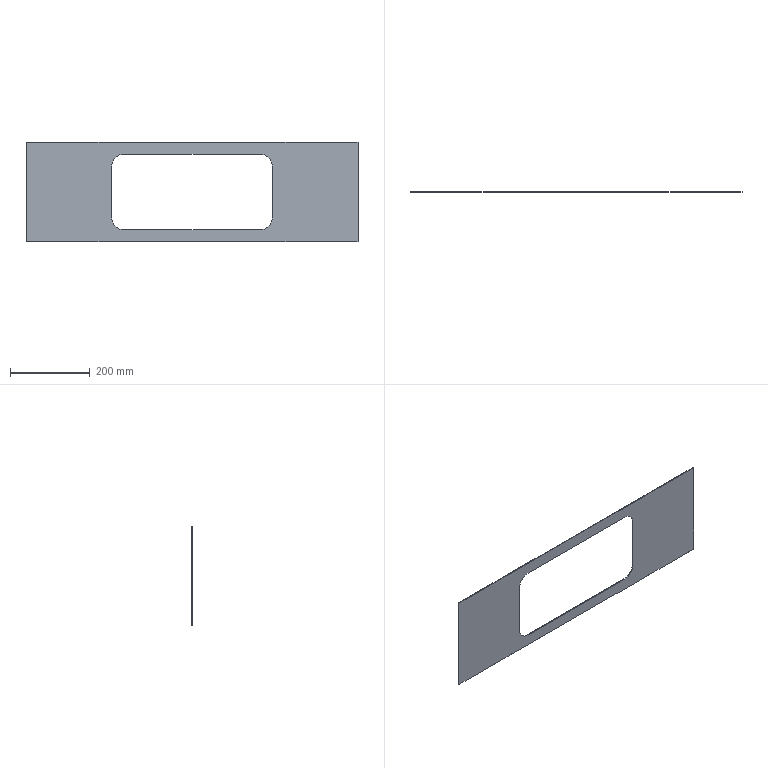Part | STEP file | Control Box Lower Base 2 | 1 solid | 46 faces | box 832.569 x 2 x 250 mm | volume 265061 mm3 | plane 42 | cylinder 4 | commonest cylinder face diameters 60 x4
STEP:
#1=CARTESIAN_POINT('',(422.364,0.,250.));
#2=VERTEX_POINT('',#1);
#3=CARTESIAN_POINT('',(422.364,0.,249.));
#4=VERTEX_POINT('',#3);
#5=CARTESIAN_POINT('',(422.364,0.,249.));
#6=DIRECTION('',(0.,0.,-1.));
#7=VECTOR('',#6,1000.);
#8=LINE('',#5,#7);
#9=EDGE_CURVE('',#2,#4,#8,.T.);
#10=ORIENTED_EDGE('',*,*,#9,.T.);
#11=CARTESIAN_POINT('',(422.864,0.,249.));
#12=VERTEX_POINT('',#11);
#13=CARTESIAN_POINT('',(422.364,0.,249.));
#14=DIRECTION('',(1.,0.,0.));
#15=VECTOR('',#14,1000.);
#16=LINE('',#13,#15);
#17=EDGE_CURVE('',#4,#12,#16,.T.);
#18=ORIENTED_EDGE('',*,*,#17,.T.);
#19=CARTESIAN_POINT('',(422.864,0.,250.));
#20=VERTEX_POINT('',#19);
#21=CARTESIAN_POINT('',(422.864,0.,249.));
#22=DIRECTION('',(0.,0.,1.));
#23=VECTOR('',#22,1000.);
#24=LINE('',#21,#23);
#25=EDGE_CURVE('',#12,#20,#24,.T.);
#26=ORIENTED_EDGE('',*,*,#25,.T.);
#27=CARTESIAN_POINT('',(581.864,0.,250.));
#28=VERTEX_POINT('',#27);
#29=CARTESIAN_POINT('',(396.579,0.,250.));
#30=DIRECTION('',(-1.,0.,0.));
#31=VECTOR('',#30,1000.);
#32=LINE('',#29,#31);
#33=EDGE_CURVE('',#28,#20,#32,.T.);
#34=ORIENTED_EDGE('',*,*,#33,.F.);
#35=CARTESIAN_POINT('',(581.864,0.,0.));
#36=VERTEX_POINT('',#35);
#37=CARTESIAN_POINT('',(581.864,0.,250.));
#38=DIRECTION('',(0.,0.,1.));
#39=VECTOR('',#38,1000.);
#40=LINE('',#37,#39);
#41=EDGE_CURVE('',#36,#28,#40,.T.);
#42=ORIENTED_EDGE('',*,*,#41,.F.);
#43=CARTESIAN_POINT('',(422.864,0.,0.));
#44=VERTEX_POINT('',#43);
#45=CARTESIAN_POINT('',(396.579,0.,0.));
#46=DIRECTION('',(1.,0.,0.));
#47=VECTOR('',#46,1000.);
#48=LINE('',#45,#47);
#49=EDGE_CURVE('',#44,#36,#48,.T.);
#50=ORIENTED_EDGE('',*,*,#49,.F.);
#51=CARTESIAN_POINT('',(422.864,0.,1.));
#52=VERTEX_POINT('',#51);
#53=CARTESIAN_POINT('',(422.864,0.,0.));
#54=DIRECTION('',(0.,0.,1.));
#55=VECTOR('',#54,1000.);
#56=LINE('',#53,#55);
#57=EDGE_CURVE('',#44,#52,#56,.T.);
#58=ORIENTED_EDGE('',*,*,#57,.T.);
#59=CARTESIAN_POINT('',(422.364,0.,1.));
#60=VERTEX_POINT('',#59);
#61=CARTESIAN_POINT('',(422.364,0.,1.));
#62=DIRECTION('',(-1.,0.,0.));
#63=VECTOR('',#62,1000.);
#64=LINE('',#61,#63);
#65=EDGE_CURVE('',#52,#60,#64,.T.);
#66=ORIENTED_EDGE('',*,*,#65,.T.);
#67=CARTESIAN_POINT('',(422.364,0.,0.));
#68=VERTEX_POINT('',#67);
#69=CARTESIAN_POINT('',(422.364,0.,0.));
#70=DIRECTION('',(0.,0.,-1.));
#71=VECTOR('',#70,1000.);
#72=LINE('',#69,#71);
#73=EDGE_CURVE('',#60,#68,#72,.T.);
#74=ORIENTED_EDGE('',*,*,#73,.T.);
#75=CARTESIAN_POINT('',(396.079,0.,0.));
#76=VERTEX_POINT('',#75);
#77=CARTESIAN_POINT('',(396.579,0.,0.));
#78=DIRECTION('',(1.,0.,0.));
#79=VECTOR('',#78,1000.);
#80=LINE('',#77,#79);
#81=EDGE_CURVE('',#76,#68,#80,.T.);
#82=ORIENTED_EDGE('',*,*,#81,.F.);
#83=CARTESIAN_POINT('',(396.079,0.,1.));
#84=VERTEX_POINT('',#83);
#85=CARTESIAN_POINT('',(396.079,0.,0.));
#86=DIRECTION('',(0.,0.,1.));
#87=VECTOR('',#86,1000.);
#88=LINE('',#85,#87);
#89=EDGE_CURVE('',#76,#84,#88,.T.);
#90=ORIENTED_EDGE('',*,*,#89,.T.);
#91=CARTESIAN_POINT('',(395.579,0.,1.));
#92=VERTEX_POINT('',#91);
#93=CARTESIAN_POINT('',(395.579,0.,1.));
#94=DIRECTION('',(-1.,0.,0.));
#95=VECTOR('',#94,1000.);
#96=LINE('',#93,#95);
#97=EDGE_CURVE('',#84,#92,#96,.T.);
#98=ORIENTED_EDGE('',*,*,#97,.T.);
#99=CARTESIAN_POINT('',(395.579,0.,0.));
#100=VERTEX_POINT('',#99);
#101=CARTESIAN_POINT('',(395.579,0.,0.));
#102=DIRECTION('',(0.,0.,-1.));
#103=VECTOR('',#102,1000.);
#104=LINE('',#101,#103);
#105=EDGE_CURVE('',#92,#100,#104,.T.);
#106=ORIENTED_EDGE('',*,*,#105,.T.);
#107=CARTESIAN_POINT('',(-64.421,0.,0.));
#108=VERTEX_POINT('',#107);
#109=CARTESIAN_POINT('',(396.579,0.,0.));
#110=DIRECTION('',(1.,0.,0.));
#111=VECTOR('',#110,1000.);
#112=LINE('',#109,#111);
#113=EDGE_CURVE('',#108,#100,#112,.T.);
#114=ORIENTED_EDGE('',*,*,#113,.F.);
#115=CARTESIAN_POINT('',(-64.421,0.,1.));
#116=VERTEX_POINT('',#115);
#117=CARTESIAN_POINT('',(-64.421,0.,0.));
#118=DIRECTION('',(0.,0.,1.));
#119=VECTOR('',#118,1000.);
#120=LINE('',#117,#119);
#121=EDGE_CURVE('',#108,#116,#120,.T.);
#122=ORIENTED_EDGE('',*,*,#121,.T.);
#123=CARTESIAN_POINT('',(-64.921,0.,1.));
#124=VERTEX_POINT('',#123);
#125=CARTESIAN_POINT('',(-64.921,0.,1.));
#126=DIRECTION('',(-1.,0.,0.));
#127=VECTOR('',#126,1000.);
#128=LINE('',#125,#127);
#129=EDGE_CURVE('',#116,#124,#128,.T.);
#130=ORIENTED_EDGE('',*,*,#129,.T.);
#131=CARTESIAN_POINT('',(-64.921,0.,0.));
#132=VERTEX_POINT('',#131);
#133=CARTESIAN_POINT('',(-64.921,0.,0.));
#134=DIRECTION('',(0.,0.,-1.));
#135=VECTOR('',#134,1000.);
#136=LINE('',#133,#135);
#137=EDGE_CURVE('',#124,#132,#136,.T.);
#138=ORIENTED_EDGE('',*,*,#137,.T.);
#139=CARTESIAN_POINT('',(-91.205,0.,0.));
#140=VERTEX_POINT('',#139);
#141=CARTESIAN_POINT('',(396.579,0.,0.));
#142=DIRECTION('',(1.,0.,0.));
#143=VECTOR('',#142,1000.);
#144=LINE('',#141,#143);
#145=EDGE_CURVE('',#140,#132,#144,.T.);
#146=ORIENTED_EDGE('',*,*,#145,.F.);
#147=CARTESIAN_POINT('',(-91.205,0.,1.));
#148=VERTEX_POINT('',#147);
#149=CARTESIAN_POINT('',(-91.205,0.,0.));
#150=DIRECTION('',(0.,0.,1.));
#151=VECTOR('',#150,1000.);
#152=LINE('',#149,#151);
#153=EDGE_CURVE('',#140,#148,#152,.T.);
#154=ORIENTED_EDGE('',*,*,#153,.T.);
#155=CARTESIAN_POINT('',(-91.705,0.,1.));
#156=VERTEX_POINT('',#155);
#157=CARTESIAN_POINT('',(-91.705,0.,1.));
#158=DIRECTION('',(-1.,0.,0.));
#159=VECTOR('',#158,1000.);
#160=LINE('',#157,#159);
#161=EDGE_CURVE('',#148,#156,#160,.T.);
#162=ORIENTED_EDGE('',*,*,#161,.T.);
#163=CARTESIAN_POINT('',(-91.705,0.,0.));
#164=VERTEX_POINT('',#163);
#165=CARTESIAN_POINT('',(-91.705,0.,0.));
#166=DIRECTION('',(0.,0.,-1.));
#167=VECTOR('',#166,1000.);
#168=LINE('',#165,#167);
#169=EDGE_CURVE('',#156,#164,#168,.T.);
#170=ORIENTED_EDGE('',*,*,#169,.T.);
#171=CARTESIAN_POINT('',(-250.705,0.,0.));
#172=VERTEX_POINT('',#171);
#173=CARTESIAN_POINT('',(396.579,0.,0.));
#174=DIRECTION('',(1.,0.,0.));
#175=VECTOR('',#174,1000.);
#176=LINE('',#173,#175);
#177=EDGE_CURVE('',#172,#164,#176,.T.);
#178=ORIENTED_EDGE('',*,*,#177,.F.);
#179=CARTESIAN_POINT('',(-250.705,0.,250.));
#180=VERTEX_POINT('',#179);
#181=CARTESIAN_POINT('',(-250.705,0.,250.));
#182=DIRECTION('',(0.,0.,-1.));
#183=VECTOR('',#182,1000.);
#184=LINE('',#181,#183);
#185=EDGE_CURVE('',#180,#172,#184,.T.);
#186=ORIENTED_EDGE('',*,*,#185,.F.);
#187=CARTESIAN_POINT('',(-91.705,0.,250.));
#188=VERTEX_POINT('',#187);
#189=CARTESIAN_POINT('',(396.579,0.,250.));
#190=DIRECTION('',(-1.,0.,0.));
#191=VECTOR('',#190,1000.);
#192=LINE('',#189,#191);
#193=EDGE_CURVE('',#188,#180,#192,.T.);
#194=ORIENTED_EDGE('',*,*,#193,.F.);
#195=CARTESIAN_POINT('',(-91.705,0.,249.));
#196=VERTEX_POINT('',#195);
#197=CARTESIAN_POINT('',(-91.705,0.,249.));
#198=DIRECTION('',(0.,0.,-1.));
#199=VECTOR('',#198,1000.);
#200=LINE('',#197,#199);
#201=EDGE_CURVE('',#188,#196,#200,.T.);
#202=ORIENTED_EDGE('',*,*,#201,.T.);
#203=CARTESIAN_POINT('',(-91.205,0.,249.));
#204=VERTEX_POINT('',#203);
#205=CARTESIAN_POINT('',(-91.705,0.,249.));
#206=DIRECTION('',(1.,0.,0.));
#207=VECTOR('',#206,1000.);
#208=LINE('',#205,#207);
#209=EDGE_CURVE('',#196,#204,#208,.T.);
#210=ORIENTED_EDGE('',*,*,#209,.T.);
#211=CARTESIAN_POINT('',(-91.205,0.,250.));
#212=VERTEX_POINT('',#211);
#213=CARTESIAN_POINT('',(-91.205,0.,249.));
#214=DIRECTION('',(0.,0.,1.));
#215=VECTOR('',#214,1000.);
#216=LINE('',#213,#215);
#217=EDGE_CURVE('',#204,#212,#216,.T.);
#218=ORIENTED_EDGE('',*,*,#217,.T.);
#219=CARTESIAN_POINT('',(-64.921,0.,250.));
#220=VERTEX_POINT('',#219);
#221=CARTESIAN_POINT('',(396.579,0.,250.));
#222=DIRECTION('',(-1.,0.,0.));
#223=VECTOR('',#222,1000.);
#224=LINE('',#221,#223);
#225=EDGE_CURVE('',#220,#212,#224,.T.);
#226=ORIENTED_EDGE('',*,*,#225,.F.);
#227=CARTESIAN_POINT('',(-64.921,0.,249.));
#228=VERTEX_POINT('',#227);
#229=CARTESIAN_POINT('',(-64.921,0.,249.));
#230=DIRECTION('',(0.,0.,-1.));
#231=VECTOR('',#230,1000.);
#232=LINE('',#229,#231);
#233=EDGE_CURVE('',#220,#228,#232,.T.);
#234=ORIENTED_EDGE('',*,*,#233,.T.);
#235=CARTESIAN_POINT('',(-64.421,0.,249.));
#236=VERTEX_POINT('',#235);
#237=CARTESIAN_POINT('',(-64.921,0.,249.));
#238=DIRECTION('',(1.,0.,0.));
#239=VECTOR('',#238,1000.);
#240=LINE('',#237,#239);
#241=EDGE_CURVE('',#228,#236,#240,.T.);
#242=ORIENTED_EDGE('',*,*,#241,.T.);
#243=CARTESIAN_POINT('',(-64.421,0.,250.));
#244=VERTEX_POINT('',#243);
#245=CARTESIAN_POINT('',(-64.421,0.,249.));
#246=DIRECTION('',(0.,0.,1.));
#247=VECTOR('',#246,1000.);
#248=LINE('',#245,#247);
#249=EDGE_CURVE('',#236,#244,#248,.T.);
#250=ORIENTED_EDGE('',*,*,#249,.T.);
#251=CARTESIAN_POINT('',(395.579,0.,250.));
#252=VERTEX_POINT('',#251);
#253=CARTESIAN_POINT('',(396.579,0.,250.));
#254=DIRECTION('',(-1.,0.,0.));
#255=VECTOR('',#254,1000.);
#256=LINE('',#253,#255);
#257=EDGE_CURVE('',#252,#244,#256,.T.);
#258=ORIENTED_EDGE('',*,*,#257,.F.);
#259=CARTESIAN_POINT('',(395.579,0.,249.));
#260=VERTEX_POINT('',#259);
#261=CARTESIAN_POINT('',(395.579,0.,249.));
#262=DIRECTION('',(0.,0.,-1.));
#263=VECTOR('',#262,1000.);
#264=LINE('',#261,#263);
#265=EDGE_CURVE('',#252,#260,#264,.T.);
#266=ORIENTED_EDGE('',*,*,#265,.T.);
#267=CARTESIAN_POINT('',(396.079,0.,249.));
#268=VERTEX_POINT('',#267);
#269=CARTESIAN_POINT('',(395.579,0.,249.));
#270=DIRECTION('',(1.,0.,0.));
#271=VECTOR('',#270,1000.);
#272=LINE('',#269,#271);
#273=EDGE_CURVE('',#260,#268,#272,.T.);
#274=ORIENTED_EDGE('',*,*,#273,.T.);
#275=CARTESIAN_POINT('',(396.079,0.,250.));
#276=VERTEX_POINT('',#275);
#277=CARTESIAN_POINT('',(396.079,0.,249.));
#278=DIRECTION('',(0.,0.,1.));
#279=VECTOR('',#278,1000.);
#280=LINE('',#277,#279);
#281=EDGE_CURVE('',#268,#276,#280,.T.);
#282=ORIENTED_EDGE('',*,*,#281,.T.);
#283=CARTESIAN_POINT('',(396.579,0.,250.));
#284=DIRECTION('',(-1.,0.,0.));
#285=VECTOR('',#284,1000.);
#286=LINE('',#283,#285);
#287=EDGE_CURVE('',#2,#276,#286,.T.);
#288=ORIENTED_EDGE('',*,*,#287,.F.);
#289=EDGE_LOOP('',(#10,#18,#26,#34,#42,#50,#58,#66,#74,#82,#90,#98,#106,#114,#122,#130,#138,#146,#154,#162,#170,#178,#186,#194,#202,#210,#218,#226,#234,#242,#250,#258,#266,#274,#282,#288));
#290=FACE_OUTER_BOUND('',#289,.T.);
#291=CARTESIAN_POINT('',(-35.421,0.,190.));
#292=VERTEX_POINT('',#291);
#293=CARTESIAN_POINT('',(-5.421,0.,220.));
#294=VERTEX_POINT('',#293);
#295=CARTESIAN_POINT('',(-5.421,0.,190.));
#296=DIRECTION('',(0.,1.,0.));
#297=DIRECTION('',(0.,0.,1.));
#298=AXIS2_PLACEMENT_3D('',#295,#296,#297);
#299=CIRCLE('',#298,30.);
#300=EDGE_CURVE('',#292,#294,#299,.T.);
#301=ORIENTED_EDGE('',*,*,#300,.F.);
#302=CARTESIAN_POINT('',(-35.421,0.,60.));
#303=VERTEX_POINT('',#302);
#304=CARTESIAN_POINT('',(-35.421,0.,250.));
#305=DIRECTION('',(0.,0.,1.));
#306=VECTOR('',#305,1000.);
#307=LINE('',#304,#306);
#308=EDGE_CURVE('',#303,#292,#307,.T.);
#309=ORIENTED_EDGE('',*,*,#308,.F.);
#310=CARTESIAN_POINT('',(-5.421,0.,30.));
#311=VERTEX_POINT('',#310);
#312=CARTESIAN_POINT('',(-5.421,0.,60.));
#313=DIRECTION('',(0.,1.,0.));
#314=DIRECTION('',(0.,0.,1.));
#315=AXIS2_PLACEMENT_3D('',#312,#313,#314);
#316=CIRCLE('',#315,30.);
#317=EDGE_CURVE('',#311,#303,#316,.T.);
#318=ORIENTED_EDGE('',*,*,#317,.F.);
#319=CARTESIAN_POINT('',(336.579,0.,30.));
#320=VERTEX_POINT('',#319);
#321=CARTESIAN_POINT('',(396.579,0.,30.));
#322=DIRECTION('',(-1.,0.,0.));
#323=VECTOR('',#322,1000.);
#324=LINE('',#321,#323);
#325=EDGE_CURVE('',#320,#311,#324,.T.);
#326=ORIENTED_EDGE('',*,*,#325,.F.);
#327=CARTESIAN_POINT('',(366.579,0.,60.));
#328=VERTEX_POINT('',#327);
#329=CARTESIAN_POINT('',(336.579,0.,60.));
#330=DIRECTION('',(0.,1.,0.));
#331=DIRECTION('',(0.,0.,1.));
#332=AXIS2_PLACEMENT_3D('',#329,#330,#331);
#333=CIRCLE('',#332,30.);
#334=EDGE_CURVE('',#328,#320,#333,.T.);
#335=ORIENTED_EDGE('',*,*,#334,.F.);
#336=CARTESIAN_POINT('',(366.579,0.,190.));
#337=VERTEX_POINT('',#336);
#338=CARTESIAN_POINT('',(366.579,0.,250.));
#339=DIRECTION('',(0.,0.,-1.));
#340=VECTOR('',#339,1000.);
#341=LINE('',#338,#340);
#342=EDGE_CURVE('',#337,#328,#341,.T.);
#343=ORIENTED_EDGE('',*,*,#342,.F.);
#344=CARTESIAN_POINT('',(336.579,0.,220.));
#345=VERTEX_POINT('',#344);
#346=CARTESIAN_POINT('',(336.579,0.,190.));
#347=DIRECTION('',(0.,1.,0.));
#348=DIRECTION('',(0.,0.,1.));
#349=AXIS2_PLACEMENT_3D('',#346,#347,#348);
#350=CIRCLE('',#349,30.);
#351=EDGE_CURVE('',#345,#337,#350,.T.);
#352=ORIENTED_EDGE('',*,*,#351,.F.);
#353=CARTESIAN_POINT('',(396.579,0.,220.));
#354=DIRECTION('',(1.,0.,0.));
#355=VECTOR('',#354,1000.);
#356=LINE('',#353,#355);
#357=EDGE_CURVE('',#294,#345,#356,.T.);
#358=ORIENTED_EDGE('',*,*,#357,.F.);
#359=EDGE_LOOP('',(#301,#309,#318,#326,#335,#343,#352,#358));
#360=FACE_BOUND('',#359,.T.);
#361=CARTESIAN_POINT('',(396.579,0.,250.));
#362=DIRECTION('',(0.,-1.,0.));
#363=DIRECTION('',(0.,0.,-1.));
#364=AXIS2_PLACEMENT_3D('',#361,#362,#363);
#365=PLANE('',#364);
#366=ADVANCED_FACE('',(#290,#360),#365,.F.);
#367=CARTESIAN_POINT('',(396.079,-2.,250.));
#368=VERTEX_POINT('',#367);
#369=CARTESIAN_POINT('',(396.079,0.,250.));
#370=DIRECTION('',(0.,-1.,0.));
#371=VECTOR('',#370,1000.);
#372=LINE('',#369,#371);
#373=EDGE_CURVE('',#276,#368,#372,.T.);
#374=ORIENTED_EDGE('',*,*,#373,.T.);
#375=CARTESIAN_POINT('',(422.364,-2.,250.));
#376=VERTEX_POINT('',#375);
#377=CARTESIAN_POINT('',(396.579,-2.,250.));
#378=DIRECTION('',(1.,0.,0.));
#379=VECTOR('',#378,1000.);
#380=LINE('',#377,#379);
#381=EDGE_CURVE('',#368,#376,#380,.T.);
#382=ORIENTED_EDGE('',*,*,#381,.T.);
#383=CARTESIAN_POINT('',(422.364,0.,250.));
#384=DIRECTION('',(0.,1.,0.));
#385=VECTOR('',#384,1000.);
#386=LINE('',#383,#385);
#387=EDGE_CURVE('',#376,#2,#386,.T.);
#388=ORIENTED_EDGE('',*,*,#387,.T.);
#389=ORIENTED_EDGE('',*,*,#287,.T.);
#390=EDGE_LOOP('',(#374,#382,#388,#389));
#391=FACE_OUTER_BOUND('',#390,.T.);
#392=CARTESIAN_POINT('',(396.579,0.,250.));
#393=DIRECTION('',(0.,0.,1.));
#394=DIRECTION('',(1.,0.,0.));
#395=AXIS2_PLACEMENT_3D('',#392,#393,#394);
#396=PLANE('',#395);
#397=ADVANCED_FACE('',(#391),#396,.T.);
#398=CARTESIAN_POINT('',(581.864,-2.,250.));
#399=VERTEX_POINT('',#398);
#400=CARTESIAN_POINT('',(581.864,0.,250.));
#401=DIRECTION('',(0.,1.,0.));
#402=VECTOR('',#401,1000.);
#403=LINE('',#400,#402);
#404=EDGE_CURVE('',#399,#28,#403,.T.);
#405=ORIENTED_EDGE('',*,*,#404,.T.);
#406=ORIENTED_EDGE('',*,*,#33,.T.);
#407=CARTESIAN_POINT('',(422.864,-2.,250.));
#408=VERTEX_POINT('',#407);
#409=CARTESIAN_POINT('',(422.864,0.,250.));
#410=DIRECTION('',(0.,-1.,0.));
#411=VECTOR('',#410,1000.);
#412=LINE('',#409,#411);
#413=EDGE_CURVE('',#20,#408,#412,.T.);
#414=ORIENTED_EDGE('',*,*,#413,.T.);
#415=CARTESIAN_POINT('',(396.579,-2.,250.));
#416=DIRECTION('',(1.,0.,0.));
#417=VECTOR('',#416,1000.);
#418=LINE('',#415,#417);
#419=EDGE_CURVE('',#408,#399,#418,.T.);
#420=ORIENTED_EDGE('',*,*,#419,.T.);
#421=EDGE_LOOP('',(#405,#406,#414,#420));
#422=FACE_OUTER_BOUND('',#421,.T.);
#423=CARTESIAN_POINT('',(396.579,0.,250.));
#424=DIRECTION('',(0.,0.,1.));
#425=DIRECTION('',(1.,0.,0.));
#426=AXIS2_PLACEMENT_3D('',#423,#424,#425);
#427=PLANE('',#426);
#428=ADVANCED_FACE('',(#422),#427,.T.);
#429=CARTESIAN_POINT('',(581.864,-2.,0.));
#430=VERTEX_POINT('',#429);
#431=CARTESIAN_POINT('',(581.864,-2.,250.));
#432=DIRECTION('',(0.,0.,1.));
#433=VECTOR('',#432,1000.);
#434=LINE('',#431,#433);
#435=EDGE_CURVE('',#430,#399,#434,.T.);
#436=ORIENTED_EDGE('',*,*,#435,.F.);
#437=CARTESIAN_POINT('',(581.864,0.,0.));
#438=DIRECTION('',(0.,-1.,0.));
#439=VECTOR('',#438,1000.);
#440=LINE('',#437,#439);
#441=EDGE_CURVE('',#36,#430,#440,.T.);
#442=ORIENTED_EDGE('',*,*,#441,.F.);
#443=ORIENTED_EDGE('',*,*,#41,.T.);
#444=ORIENTED_EDGE('',*,*,#404,.F.);
#445=EDGE_LOOP('',(#436,#442,#443,#444));
#446=FACE_OUTER_BOUND('',#445,.T.);
#447=CARTESIAN_POINT('',(581.864,0.,250.));
#448=DIRECTION('',(-1.,0.,0.));
#449=DIRECTION('',(0.,-1.,0.));
#450=AXIS2_PLACEMENT_3D('',#447,#448,#449);
#451=PLANE('',#450);
#452=ADVANCED_FACE('',(#446),#451,.F.);
#453=ORIENTED_EDGE('',*,*,#49,.T.);
#454=ORIENTED_EDGE('',*,*,#441,.T.);
#455=CARTESIAN_POINT('',(422.864,-2.,0.));
#456=VERTEX_POINT('',#455);
#457=CARTESIAN_POINT('',(396.579,-2.,0.));
#458=DIRECTION('',(1.,0.,0.));
#459=VECTOR('',#458,1000.);
#460=LINE('',#457,#459);
#461=EDGE_CURVE('',#456,#430,#460,.T.);
#462=ORIENTED_EDGE('',*,*,#461,.F.);
#463=CARTESIAN_POINT('',(422.864,0.,0.));
#464=DIRECTION('',(0.,-1.,0.));
#465=VECTOR('',#464,1000.);
#466=LINE('',#463,#465);
#467=EDGE_CURVE('',#44,#456,#466,.T.);
#468=ORIENTED_EDGE('',*,*,#467,.F.);
#469=EDGE_LOOP('',(#453,#454,#462,#468));
#470=FACE_OUTER_BOUND('',#469,.T.);
#471=CARTESIAN_POINT('',(396.579,0.,0.));
#472=DIRECTION('',(0.,0.,1.));
#473=DIRECTION('',(1.,0.,0.));
#474=AXIS2_PLACEMENT_3D('',#471,#472,#473);
#475=PLANE('',#474);
#476=ADVANCED_FACE('',(#470),#475,.F.);
#477=CARTESIAN_POINT('',(396.079,-2.,0.));
#478=VERTEX_POINT('',#477);
#479=CARTESIAN_POINT('',(422.364,-2.,0.));
#480=VERTEX_POINT('',#479);
#481=CARTESIAN_POINT('',(396.579,-2.,0.));
#482=DIRECTION('',(1.,0.,0.));
#483=VECTOR('',#482,1000.);
#484=LINE('',#481,#483);
#485=EDGE_CURVE('',#478,#480,#484,.T.);
#486=ORIENTED_EDGE('',*,*,#485,.F.);
#487=CARTESIAN_POINT('',(396.079,0.,0.));
#488=DIRECTION('',(0.,-1.,0.));
#489=VECTOR('',#488,1000.);
#490=LINE('',#487,#489);
#491=EDGE_CURVE('',#76,#478,#490,.T.);
#492=ORIENTED_EDGE('',*,*,#491,.F.);
#493=ORIENTED_EDGE('',*,*,#81,.T.);
#494=CARTESIAN_POINT('',(422.364,0.,0.));
#495=DIRECTION('',(0.,1.,0.));
#496=VECTOR('',#495,1000.);
#497=LINE('',#494,#496);
#498=EDGE_CURVE('',#480,#68,#497,.T.);
#499=ORIENTED_EDGE('',*,*,#498,.F.);
#500=EDGE_LOOP('',(#486,#492,#493,#499));
#501=FACE_OUTER_BOUND('',#500,.T.);
#502=CARTESIAN_POINT('',(396.579,0.,0.));
#503=DIRECTION('',(0.,0.,1.));
#504=DIRECTION('',(1.,0.,0.));
#505=AXIS2_PLACEMENT_3D('',#502,#503,#504);
#506=PLANE('',#505);
#507=ADVANCED_FACE('',(#501),#506,.F.);
#508=CARTESIAN_POINT('',(-64.421,-2.,0.));
#509=VERTEX_POINT('',#508);
#510=CARTESIAN_POINT('',(395.579,-2.,0.));
#511=VERTEX_POINT('',#510);
#512=CARTESIAN_POINT('',(396.579,-2.,0.));
#513=DIRECTION('',(1.,0.,0.));
#514=VECTOR('',#513,1000.);
#515=LINE('',#512,#514);
#516=EDGE_CURVE('',#509,#511,#515,.T.);
#517=ORIENTED_EDGE('',*,*,#516,.F.);
#518=CARTESIAN_POINT('',(-64.421,0.,0.));
#519=DIRECTION('',(0.,-1.,0.));
#520=VECTOR('',#519,1000.);
#521=LINE('',#518,#520);
#522=EDGE_CURVE('',#108,#509,#521,.T.);
#523=ORIENTED_EDGE('',*,*,#522,.F.);
#524=ORIENTED_EDGE('',*,*,#113,.T.);
#525=CARTESIAN_POINT('',(395.579,0.,0.));
#526=DIRECTION('',(0.,1.,0.));
#527=VECTOR('',#526,1000.);
#528=LINE('',#525,#527);
#529=EDGE_CURVE('',#511,#100,#528,.T.);
#530=ORIENTED_EDGE('',*,*,#529,.F.);
#531=EDGE_LOOP('',(#517,#523,#524,#530));
#532=FACE_OUTER_BOUND('',#531,.T.);
#533=CARTESIAN_POINT('',(396.579,0.,0.));
#534=DIRECTION('',(0.,0.,1.));
#535=DIRECTION('',(1.,0.,0.));
#536=AXIS2_PLACEMENT_3D('',#533,#534,#535);
#537=PLANE('',#536);
#538=ADVANCED_FACE('',(#532),#537,.F.);
#539=CARTESIAN_POINT('',(-91.205,-2.,0.));
#540=VERTEX_POINT('',#539);
#541=CARTESIAN_POINT('',(-64.921,-2.,0.));
#542=VERTEX_POINT('',#541);
#543=CARTESIAN_POINT('',(396.579,-2.,0.));
#544=DIRECTION('',(1.,0.,0.));
#545=VECTOR('',#544,1000.);
#546=LINE('',#543,#545);
#547=EDGE_CURVE('',#540,#542,#546,.T.);
#548=ORIENTED_EDGE('',*,*,#547,.F.);
#549=CARTESIAN_POINT('',(-91.205,0.,0.));
#550=DIRECTION('',(0.,-1.,0.));
#551=VECTOR('',#550,1000.);
#552=LINE('',#549,#551);
#553=EDGE_CURVE('',#140,#540,#552,.T.);
#554=ORIENTED_EDGE('',*,*,#553,.F.);
#555=ORIENTED_EDGE('',*,*,#145,.T.);
#556=CARTESIAN_POINT('',(-64.921,0.,0.));
#557=DIRECTION('',(0.,1.,0.));
#558=VECTOR('',#557,1000.);
#559=LINE('',#556,#558);
#560=EDGE_CURVE('',#542,#132,#559,.T.);
#561=ORIENTED_EDGE('',*,*,#560,.F.);
#562=EDGE_LOOP('',(#548,#554,#555,#561));
#563=FACE_OUTER_BOUND('',#562,.T.);
#564=CARTESIAN_POINT('',(396.579,0.,0.));
#565=DIRECTION('',(0.,0.,1.));
#566=DIRECTION('',(1.,0.,0.));
#567=AXIS2_PLACEMENT_3D('',#564,#565,#566);
#568=PLANE('',#567);
#569=ADVANCED_FACE('',(#563),#568,.F.);
#570=CARTESIAN_POINT('',(-250.705,-2.,0.));
#571=VERTEX_POINT('',#570);
#572=CARTESIAN_POINT('',(-91.705,-2.,0.));
#573=VERTEX_POINT('',#572);
#574=CARTESIAN_POINT('',(396.579,-2.,0.));
#575=DIRECTION('',(1.,0.,0.));
#576=VECTOR('',#575,1000.);
#577=LINE('',#574,#576);
#578=EDGE_CURVE('',#571,#573,#577,.T.);
#579=ORIENTED_EDGE('',*,*,#578,.F.);
#580=CARTESIAN_POINT('',(-250.705,0.,0.));
#581=DIRECTION('',(0.,-1.,0.));
#582=VECTOR('',#581,1000.);
#583=LINE('',#580,#582);
#584=EDGE_CURVE('',#172,#571,#583,.T.);
#585=ORIENTED_EDGE('',*,*,#584,.F.);
#586=ORIENTED_EDGE('',*,*,#177,.T.);
#587=CARTESIAN_POINT('',(-91.705,0.,0.));
#588=DIRECTION('',(0.,1.,0.));
#589=VECTOR('',#588,1000.);
#590=LINE('',#587,#589);
#591=EDGE_CURVE('',#573,#164,#590,.T.);
#592=ORIENTED_EDGE('',*,*,#591,.F.);
#593=EDGE_LOOP('',(#579,#585,#586,#592));
#594=FACE_OUTER_BOUND('',#593,.T.);
#595=CARTESIAN_POINT('',(396.579,0.,0.));
#596=DIRECTION('',(0.,0.,1.));
#597=DIRECTION('',(1.,0.,0.));
#598=AXIS2_PLACEMENT_3D('',#595,#596,#597);
#599=PLANE('',#598);
#600=ADVANCED_FACE('',(#594),#599,.F.);
#601=CARTESIAN_POINT('',(-250.705,-2.,250.));
#602=VERTEX_POINT('',#601);
#603=CARTESIAN_POINT('',(-250.705,0.,250.));
#604=DIRECTION('',(0.,1.,0.));
#605=VECTOR('',#604,1000.);
#606=LINE('',#603,#605);
#607=EDGE_CURVE('',#602,#180,#606,.T.);
#608=ORIENTED_EDGE('',*,*,#607,.T.);
#609=ORIENTED_EDGE('',*,*,#185,.T.);
#610=ORIENTED_EDGE('',*,*,#584,.T.);
#611=CARTESIAN_POINT('',(-250.705,-2.,250.));
#612=DIRECTION('',(0.,0.,1.));
#613=VECTOR('',#612,1000.);
#614=LINE('',#611,#613);
#615=EDGE_CURVE('',#571,#602,#614,.T.);
#616=ORIENTED_EDGE('',*,*,#615,.T.);
#617=EDGE_LOOP('',(#608,#609,#610,#616));
#618=FACE_OUTER_BOUND('',#617,.T.);
#619=CARTESIAN_POINT('',(-250.705,0.,250.));
#620=DIRECTION('',(-1.,0.,0.));
#621=DIRECTION('',(0.,0.,1.));
#622=AXIS2_PLACEMENT_3D('',#619,#620,#621);
#623=PLANE('',#622);
#624=ADVANCED_FACE('',(#618),#623,.T.);
#625=ORIENTED_EDGE('',*,*,#607,.F.);
#626=CARTESIAN_POINT('',(-91.705,-2.,250.));
#627=VERTEX_POINT('',#626);
#628=CARTESIAN_POINT('',(396.579,-2.,250.));
#629=DIRECTION('',(1.,0.,0.));
#630=VECTOR('',#629,1000.);
#631=LINE('',#628,#630);
#632=EDGE_CURVE('',#602,#627,#631,.T.);
#633=ORIENTED_EDGE('',*,*,#632,.T.);
#634=CARTESIAN_POINT('',(-91.705,0.,250.));
#635=DIRECTION('',(0.,1.,0.));
#636=VECTOR('',#635,1000.);
#637=LINE('',#634,#636);
#638=EDGE_CURVE('',#627,#188,#637,.T.);
#639=ORIENTED_EDGE('',*,*,#638,.T.);
#640=ORIENTED_EDGE('',*,*,#193,.T.);
#641=EDGE_LOOP('',(#625,#633,#639,#640));
#642=FACE_OUTER_BOUND('',#641,.T.);
#643=CARTESIAN_POINT('',(396.579,0.,250.));
#644=DIRECTION('',(0.,0.,1.));
#645=DIRECTION('',(1.,0.,0.));
#646=AXIS2_PLACEMENT_3D('',#643,#644,#645);
#647=PLANE('',#646);
#648=ADVANCED_FACE('',(#642),#647,.T.);
#649=CARTESIAN_POINT('',(-91.205,-2.,250.));
#650=VERTEX_POINT('',#649);
#651=CARTESIAN_POINT('',(-91.205,0.,250.));
#652=DIRECTION('',(0.,-1.,0.));
#653=VECTOR('',#652,1000.);
#654=LINE('',#651,#653);
#655=EDGE_CURVE('',#212,#650,#654,.T.);
#656=ORIENTED_EDGE('',*,*,#655,.T.);
#657=CARTESIAN_POINT('',(-64.921,-2.,250.));
#658=VERTEX_POINT('',#657);
#659=CARTESIAN_POINT('',(396.579,-2.,250.));
#660=DIRECTION('',(1.,0.,0.));
#661=VECTOR('',#660,1000.);
#662=LINE('',#659,#661);
#663=EDGE_CURVE('',#650,#658,#662,.T.);
#664=ORIENTED_EDGE('',*,*,#663,.T.);
#665=CARTESIAN_POINT('',(-64.921,0.,250.));
#666=DIRECTION('',(0.,1.,0.));
#667=VECTOR('',#666,1000.);
#668=LINE('',#665,#667);
#669=EDGE_CURVE('',#658,#220,#668,.T.);
#670=ORIENTED_EDGE('',*,*,#669,.T.);
#671=ORIENTED_EDGE('',*,*,#225,.T.);
#672=EDGE_LOOP('',(#656,#664,#670,#671));
#673=FACE_OUTER_BOUND('',#672,.T.);
#674=CARTESIAN_POINT('',(396.579,0.,250.));
#675=DIRECTION('',(0.,0.,1.));
#676=DIRECTION('',(1.,0.,0.));
#677=AXIS2_PLACEMENT_3D('',#674,#675,#676);
#678=PLANE('',#677);
#679=ADVANCED_FACE('',(#673),#678,.T.);
#680=CARTESIAN_POINT('',(-64.421,-2.,250.));
#681=VERTEX_POINT('',#680);
#682=CARTESIAN_POINT('',(-64.421,0.,250.));
#683=DIRECTION('',(0.,-1.,0.));
#684=VECTOR('',#683,1000.);
#685=LINE('',#682,#684);
#686=EDGE_CURVE('',#244,#681,#685,.T.);
#687=ORIENTED_EDGE('',*,*,#686,.T.);
#688=CARTESIAN_POINT('',(395.579,-2.,250.));
#689=VERTEX_POINT('',#688);
#690=CARTESIAN_POINT('',(396.579,-2.,250.));
#691=DIRECTION('',(1.,0.,0.));
#692=VECTOR('',#691,1000.);
#693=LINE('',#690,#692);
#694=EDGE_CURVE('',#681,#689,#693,.T.);
#695=ORIENTED_EDGE('',*,*,#694,.T.);
#696=CARTESIAN_POINT('',(395.579,0.,250.));
#697=DIRECTION('',(0.,1.,0.));
#698=VECTOR('',#697,1000.);
#699=LINE('',#696,#698);
#700=EDGE_CURVE('',#689,#252,#699,.T.);
#701=ORIENTED_EDGE('',*,*,#700,.T.);
#702=ORIENTED_EDGE('',*,*,#257,.T.);
#703=EDGE_LOOP('',(#687,#695,#701,#702));
#704=FACE_OUTER_BOUND('',#703,.T.);
#705=CARTESIAN_POINT('',(396.579,0.,250.));
#706=DIRECTION('',(0.,0.,1.));
#707=DIRECTION('',(1.,0.,0.));
#708=AXIS2_PLACEMENT_3D('',#705,#706,#707);
#709=PLANE('',#708);
#710=ADVANCED_FACE('',(#704),#709,.T.);
#711=CARTESIAN_POINT('',(-5.421,-2.,220.));
#712=VERTEX_POINT('',#711);
#713=CARTESIAN_POINT('',(-5.421,0.,220.));
#714=DIRECTION('',(0.,1.,0.));
#715=VECTOR('',#714,1000.);
#716=LINE('',#713,#715);
#717=EDGE_CURVE('',#712,#294,#716,.T.);
#718=ORIENTED_EDGE('',*,*,#717,.T.);
#719=ORIENTED_EDGE('',*,*,#357,.T.);
#720=CARTESIAN_POINT('',(336.579,-2.,220.));
#721=VERTEX_POINT('',#720);
#722=CARTESIAN_POINT('',(336.579,0.,220.));
#723=DIRECTION('',(0.,-1.,0.));
#724=VECTOR('',#723,1000.);
#725=LINE('',#722,#724);
#726=EDGE_CURVE('',#345,#721,#725,.T.);
#727=ORIENTED_EDGE('',*,*,#726,.T.);
#728=CARTESIAN_POINT('',(-5.421,-2.,220.));
#729=DIRECTION('',(-1.,0.,0.));
#730=VECTOR('',#729,1000.);
#731=LINE('',#728,#730);
#732=EDGE_CURVE('',#721,#712,#731,.T.);
#733=ORIENTED_EDGE('',*,*,#732,.T.);
#734=EDGE_LOOP('',(#718,#719,#727,#733));
#735=FACE_OUTER_BOUND('',#734,.T.);
#736=CARTESIAN_POINT('',(-5.421,0.,220.));
#737=DIRECTION('',(0.,0.,-1.));
#738=DIRECTION('',(-1.,0.,0.));
#739=AXIS2_PLACEMENT_3D('',#736,#737,#738);
#740=PLANE('',#739);
#741=ADVANCED_FACE('',(#735),#740,.T.);
#742=CARTESIAN_POINT('',(-35.421,-2.,190.));
#743=VERTEX_POINT('',#742);
#744=CARTESIAN_POINT('',(-35.421,0.,190.));
#745=DIRECTION('',(0.,-1.,0.));
#746=VECTOR('',#745,1000.);
#747=LINE('',#744,#746);
#748=EDGE_CURVE('',#292,#743,#747,.T.);
#749=ORIENTED_EDGE('',*,*,#748,.F.);
#750=ORIENTED_EDGE('',*,*,#300,.T.);
#751=ORIENTED_EDGE('',*,*,#717,.F.);
#752=CARTESIAN_POINT('',(-5.421,-2.,190.));
#753=DIRECTION('',(0.,1.,0.));
#754=DIRECTION('',(0.,0.,1.));
#755=AXIS2_PLACEMENT_3D('',#752,#753,#754);
#756=CIRCLE('',#755,30.);
#757=EDGE_CURVE('',#743,#712,#756,.T.);
#758=ORIENTED_EDGE('',*,*,#757,.F.);
#759=EDGE_LOOP('',(#749,#750,#751,#758));
#760=FACE_OUTER_BOUND('',#759,.T.);
#761=CARTESIAN_POINT('',(-5.421,0.,190.));
#762=DIRECTION('',(0.,1.,0.));
#763=DIRECTION('',(0.,0.,1.));
#764=AXIS2_PLACEMENT_3D('',#761,#762,#763);
#765=CYLINDRICAL_SURFACE('',#764,30.);
#766=ADVANCED_FACE('',(#760),#765,.F.);
#767=CARTESIAN_POINT('',(-35.421,-2.,60.));
#768=VERTEX_POINT('',#767);
#769=CARTESIAN_POINT('',(-35.421,0.,60.));
#770=DIRECTION('',(0.,1.,0.));
#771=VECTOR('',#770,1000.);
#772=LINE('',#769,#771);
#773=EDGE_CURVE('',#768,#303,#772,.T.);
#774=ORIENTED_EDGE('',*,*,#773,.T.);
#775=ORIENTED_EDGE('',*,*,#308,.T.);
#776=ORIENTED_EDGE('',*,*,#748,.T.);
#777=CARTESIAN_POINT('',(-35.421,-2.,60.));
#778=DIRECTION('',(0.,0.,-1.));
#779=VECTOR('',#778,1000.);
#780=LINE('',#777,#779);
#781=EDGE_CURVE('',#743,#768,#780,.T.);
#782=ORIENTED_EDGE('',*,*,#781,.T.);
#783=EDGE_LOOP('',(#774,#775,#776,#782));
#784=FACE_OUTER_BOUND('',#783,.T.);
#785=CARTESIAN_POINT('',(-35.421,0.,60.));
#786=DIRECTION('',(1.,0.,0.));
#787=DIRECTION('',(0.,0.,-1.));
#788=AXIS2_PLACEMENT_3D('',#785,#786,#787);
#789=PLANE('',#788);
#790=ADVANCED_FACE('',(#784),#789,.T.);
#791=CARTESIAN_POINT('',(-5.421,-2.,30.));
#792=VERTEX_POINT('',#791);
#793=CARTESIAN_POINT('',(-5.421,-2.,60.));
#794=DIRECTION('',(0.,1.,0.));
#795=DIRECTION('',(0.,0.,1.));
#796=AXIS2_PLACEMENT_3D('',#793,#794,#795);
#797=CIRCLE('',#796,30.);
#798=EDGE_CURVE('',#792,#768,#797,.T.);
#799=ORIENTED_EDGE('',*,*,#798,.F.);
#800=CARTESIAN_POINT('',(-5.421,0.,30.));
#801=DIRECTION('',(0.,-1.,0.));
#802=VECTOR('',#801,1000.);
#803=LINE('',#800,#802);
#804=EDGE_CURVE('',#311,#792,#803,.T.);
#805=ORIENTED_EDGE('',*,*,#804,.F.);
#806=ORIENTED_EDGE('',*,*,#317,.T.);
#807=ORIENTED_EDGE('',*,*,#773,.F.);
#808=EDGE_LOOP('',(#799,#805,#806,#807));
#809=FACE_OUTER_BOUND('',#808,.T.);
#810=CARTESIAN_POINT('',(-5.421,0.,60.));
#811=DIRECTION('',(0.,1.,0.));
#812=DIRECTION('',(0.,0.,1.));
#813=AXIS2_PLACEMENT_3D('',#810,#811,#812);
#814=CYLINDRICAL_SURFACE('',#813,30.);
#815=ADVANCED_FACE('',(#809),#814,.F.);
#816=CARTESIAN_POINT('',(336.579,-2.,30.));
#817=VERTEX_POINT('',#816);
#818=CARTESIAN_POINT('',(336.579,0.,30.));
#819=DIRECTION('',(0.,1.,0.));
#820=VECTOR('',#819,1000.);
#821=LINE('',#818,#820);
#822=EDGE_CURVE('',#817,#320,#821,.T.);
#823=ORIENTED_EDGE('',*,*,#822,.T.);
#824=ORIENTED_EDGE('',*,*,#325,.T.);
#825=ORIENTED_EDGE('',*,*,#804,.T.);
#826=CARTESIAN_POINT('',(336.579,-2.,30.));
#827=DIRECTION('',(1.,0.,0.));
#828=VECTOR('',#827,1000.);
#829=LINE('',#826,#828);
#830=EDGE_CURVE('',#792,#817,#829,.T.);
#831=ORIENTED_EDGE('',*,*,#830,.T.);
#832=EDGE_LOOP('',(#823,#824,#825,#831));
#833=FACE_OUTER_BOUND('',#832,.T.);
#834=CARTESIAN_POINT('',(336.579,0.,30.));
#835=DIRECTION('',(0.,0.,1.));
#836=DIRECTION('',(1.,0.,0.));
#837=AXIS2_PLACEMENT_3D('',#834,#835,#836);
#838=PLANE('',#837);
#839=ADVANCED_FACE('',(#833),#838,.T.);
#840=CARTESIAN_POINT('',(366.579,-2.,60.));
#841=VERTEX_POINT('',#840);
#842=CARTESIAN_POINT('',(336.579,-2.,60.));
#843=DIRECTION('',(0.,1.,0.));
#844=DIRECTION('',(0.,0.,1.));
#845=AXIS2_PLACEMENT_3D('',#842,#843,#844);
#846=CIRCLE('',#845,30.);
#847=EDGE_CURVE('',#841,#817,#846,.T.);
#848=ORIENTED_EDGE('',*,*,#847,.F.);
#849=CARTESIAN_POINT('',(366.579,0.,60.));
#850=DIRECTION('',(0.,-1.,0.));
#851=VECTOR('',#850,1000.);
#852=LINE('',#849,#851);
#853=EDGE_CURVE('',#328,#841,#852,.T.);
#854=ORIENTED_EDGE('',*,*,#853,.F.);
#855=ORIENTED_EDGE('',*,*,#334,.T.);
#856=ORIENTED_EDGE('',*,*,#822,.F.);
#857=EDGE_LOOP('',(#848,#854,#855,#856));
#858=FACE_OUTER_BOUND('',#857,.T.);
#859=CARTESIAN_POINT('',(336.579,0.,60.));
#860=DIRECTION('',(0.,1.,0.));
#861=DIRECTION('',(0.,0.,1.));
#862=AXIS2_PLACEMENT_3D('',#859,#860,#861);
#863=CYLINDRICAL_SURFACE('',#862,30.);
#864=ADVANCED_FACE('',(#858),#863,.F.);
#865=CARTESIAN_POINT('',(366.579,-2.,190.));
#866=VERTEX_POINT('',#865);
#867=CARTESIAN_POINT('',(366.579,0.,190.));
#868=DIRECTION('',(0.,1.,0.));
#869=VECTOR('',#868,1000.);
#870=LINE('',#867,#869);
#871=EDGE_CURVE('',#866,#337,#870,.T.);
#872=ORIENTED_EDGE('',*,*,#871,.T.);
#873=ORIENTED_EDGE('',*,*,#342,.T.);
#874=ORIENTED_EDGE('',*,*,#853,.T.);
#875=CARTESIAN_POINT('',(366.579,-2.,190.));
#876=DIRECTION('',(0.,0.,1.));
#877=VECTOR('',#876,1000.);
#878=LINE('',#875,#877);
#879=EDGE_CURVE('',#841,#866,#878,.T.);
#880=ORIENTED_EDGE('',*,*,#879,.T.);
#881=EDGE_LOOP('',(#872,#873,#874,#880));
#882=FACE_OUTER_BOUND('',#881,.T.);
#883=CARTESIAN_POINT('',(366.579,0.,190.));
#884=DIRECTION('',(-1.,0.,0.));
#885=DIRECTION('',(0.,0.,1.));
#886=AXIS2_PLACEMENT_3D('',#883,#884,#885);
#887=PLANE('',#886);
#888=ADVANCED_FACE('',(#882),#887,.T.);
#889=CARTESIAN_POINT('',(336.579,-2.,190.));
#890=DIRECTION('',(0.,1.,0.));
#891=DIRECTION('',(0.,0.,1.));
#892=AXIS2_PLACEMENT_3D('',#889,#890,#891);
#893=CIRCLE('',#892,30.);
#894=EDGE_CURVE('',#721,#866,#893,.T.);
#895=ORIENTED_EDGE('',*,*,#894,.F.);
#896=ORIENTED_EDGE('',*,*,#726,.F.);
#897=ORIENTED_EDGE('',*,*,#351,.T.);
#898=ORIENTED_EDGE('',*,*,#871,.F.);
#899=EDGE_LOOP('',(#895,#896,#897,#898));
#900=FACE_OUTER_BOUND('',#899,.T.);
#901=CARTESIAN_POINT('',(336.579,0.,190.));
#902=DIRECTION('',(0.,1.,0.));
#903=DIRECTION('',(0.,0.,1.));
#904=AXIS2_PLACEMENT_3D('',#901,#902,#903);
#905=CYLINDRICAL_SURFACE('',#904,30.);
#906=ADVANCED_FACE('',(#900),#905,.F.);
#907=ORIENTED_EDGE('',*,*,#781,.F.);
#908=ORIENTED_EDGE('',*,*,#757,.T.);
#909=ORIENTED_EDGE('',*,*,#732,.F.);
#910=ORIENTED_EDGE('',*,*,#894,.T.);
#911=ORIENTED_EDGE('',*,*,#879,.F.);
#912=ORIENTED_EDGE('',*,*,#847,.T.);
#913=ORIENTED_EDGE('',*,*,#830,.F.);
#914=ORIENTED_EDGE('',*,*,#798,.T.);
#915=EDGE_LOOP('',(#907,#908,#909,#910,#911,#912,#913,#914));
#916=FACE_BOUND('',#915,.T.);
#917=CARTESIAN_POINT('',(422.864,-2.,249.));
#918=VERTEX_POINT('',#917);
#919=CARTESIAN_POINT('',(422.864,-2.,250.));
#920=DIRECTION('',(0.,0.,-1.));
#921=VECTOR('',#920,1000.);
#922=LINE('',#919,#921);
#923=EDGE_CURVE('',#408,#918,#922,.T.);
#924=ORIENTED_EDGE('',*,*,#923,.T.);
#925=CARTESIAN_POINT('',(422.364,-2.,249.));
#926=VERTEX_POINT('',#925);
#927=CARTESIAN_POINT('',(422.364,-2.,249.));
#928=DIRECTION('',(-1.,0.,0.));
#929=VECTOR('',#928,1000.);
#930=LINE('',#927,#929);
#931=EDGE_CURVE('',#918,#926,#930,.T.);
#932=ORIENTED_EDGE('',*,*,#931,.T.);
#933=CARTESIAN_POINT('',(422.364,-2.,250.));
#934=DIRECTION('',(0.,0.,1.));
#935=VECTOR('',#934,1000.);
#936=LINE('',#933,#935);
#937=EDGE_CURVE('',#926,#376,#936,.T.);
#938=ORIENTED_EDGE('',*,*,#937,.T.);
#939=ORIENTED_EDGE('',*,*,#381,.F.);
#940=CARTESIAN_POINT('',(396.079,-2.,249.));
#941=VERTEX_POINT('',#940);
#942=CARTESIAN_POINT('',(396.079,-2.,250.));
#943=DIRECTION('',(0.,0.,-1.));
#944=VECTOR('',#943,1000.);
#945=LINE('',#942,#944);
#946=EDGE_CURVE('',#368,#941,#945,.T.);
#947=ORIENTED_EDGE('',*,*,#946,.T.);
#948=CARTESIAN_POINT('',(395.579,-2.,249.));
#949=VERTEX_POINT('',#948);
#950=CARTESIAN_POINT('',(395.579,-2.,249.));
#951=DIRECTION('',(-1.,0.,0.));
#952=VECTOR('',#951,1000.);
#953=LINE('',#950,#952);
#954=EDGE_CURVE('',#941,#949,#953,.T.);
#955=ORIENTED_EDGE('',*,*,#954,.T.);
#956=CARTESIAN_POINT('',(395.579,-2.,250.));
#957=DIRECTION('',(0.,0.,1.));
#958=VECTOR('',#957,1000.);
#959=LINE('',#956,#958);
#960=EDGE_CURVE('',#949,#689,#959,.T.);
#961=ORIENTED_EDGE('',*,*,#960,.T.);
#962=ORIENTED_EDGE('',*,*,#694,.F.);
#963=CARTESIAN_POINT('',(-64.421,-2.,249.));
#964=VERTEX_POINT('',#963);
#965=CARTESIAN_POINT('',(-64.421,-2.,250.));
#966=DIRECTION('',(0.,0.,-1.));
#967=VECTOR('',#966,1000.);
#968=LINE('',#965,#967);
#969=EDGE_CURVE('',#681,#964,#968,.T.);
#970=ORIENTED_EDGE('',*,*,#969,.T.);
#971=CARTESIAN_POINT('',(-64.921,-2.,249.));
#972=VERTEX_POINT('',#971);
#973=CARTESIAN_POINT('',(-64.921,-2.,249.));
#974=DIRECTION('',(-1.,0.,0.));
#975=VECTOR('',#974,1000.);
#976=LINE('',#973,#975);
#977=EDGE_CURVE('',#964,#972,#976,.T.);
#978=ORIENTED_EDGE('',*,*,#977,.T.);
#979=CARTESIAN_POINT('',(-64.921,-2.,250.));
#980=DIRECTION('',(0.,0.,1.));
#981=VECTOR('',#980,1000.);
#982=LINE('',#979,#981);
#983=EDGE_CURVE('',#972,#658,#982,.T.);
#984=ORIENTED_EDGE('',*,*,#983,.T.);
#985=ORIENTED_EDGE('',*,*,#663,.F.);
#986=CARTESIAN_POINT('',(-91.205,-2.,249.));
#987=VERTEX_POINT('',#986);
#988=CARTESIAN_POINT('',(-91.205,-2.,250.));
#989=DIRECTION('',(0.,0.,-1.));
#990=VECTOR('',#989,1000.);
#991=LINE('',#988,#990);
#992=EDGE_CURVE('',#650,#987,#991,.T.);
#993=ORIENTED_EDGE('',*,*,#992,.T.);
#994=CARTESIAN_POINT('',(-91.705,-2.,249.));
#995=VERTEX_POINT('',#994);
#996=CARTESIAN_POINT('',(-91.705,-2.,249.));
#997=DIRECTION('',(-1.,0.,0.));
#998=VECTOR('',#997,1000.);
#999=LINE('',#996,#998);
#1000=EDGE_CURVE('',#987,#995,#999,.T.);
#1001=ORIENTED_EDGE('',*,*,#1000,.T.);
#1002=CARTESIAN_POINT('',(-91.705,-2.,250.));
#1003=DIRECTION('',(0.,0.,1.));
#1004=VECTOR('',#1003,1000.);
#1005=LINE('',#1002,#1004);
#1006=EDGE_CURVE('',#995,#627,#1005,.T.);
#1007=ORIENTED_EDGE('',*,*,#1006,.T.);
#1008=ORIENTED_EDGE('',*,*,#632,.F.);
#1009=ORIENTED_EDGE('',*,*,#615,.F.);
#1010=ORIENTED_EDGE('',*,*,#578,.T.);
#1011=CARTESIAN_POINT('',(-91.705,-2.,1.));
#1012=VERTEX_POINT('',#1011);
#1013=CARTESIAN_POINT('',(-91.705,-2.,250.));
#1014=DIRECTION('',(0.,0.,1.));
#1015=VECTOR('',#1014,1000.);
#1016=LINE('',#1013,#1015);
#1017=EDGE_CURVE('',#573,#1012,#1016,.T.);
#1018=ORIENTED_EDGE('',*,*,#1017,.T.);
#1019=CARTESIAN_POINT('',(-91.205,-2.,1.));
#1020=VERTEX_POINT('',#1019);
#1021=CARTESIAN_POINT('',(-91.705,-2.,1.));
#1022=DIRECTION('',(1.,0.,0.));
#1023=VECTOR('',#1022,1000.);
#1024=LINE('',#1021,#1023);
#1025=EDGE_CURVE('',#1012,#1020,#1024,.T.);
#1026=ORIENTED_EDGE('',*,*,#1025,.T.);
#1027=CARTESIAN_POINT('',(-91.205,-2.,250.));
#1028=DIRECTION('',(0.,0.,-1.));
#1029=VECTOR('',#1028,1000.);
#1030=LINE('',#1027,#1029);
#1031=EDGE_CURVE('',#1020,#540,#1030,.T.);
#1032=ORIENTED_EDGE('',*,*,#1031,.T.);
#1033=ORIENTED_EDGE('',*,*,#547,.T.);
#1034=CARTESIAN_POINT('',(-64.921,-2.,1.));
#1035=VERTEX_POINT('',#1034);
#1036=CARTESIAN_POINT('',(-64.921,-2.,250.));
#1037=DIRECTION('',(0.,0.,1.));
#1038=VECTOR('',#1037,1000.);
#1039=LINE('',#1036,#1038);
#1040=EDGE_CURVE('',#542,#1035,#1039,.T.);
#1041=ORIENTED_EDGE('',*,*,#1040,.T.);
#1042=CARTESIAN_POINT('',(-64.421,-2.,1.));
#1043=VERTEX_POINT('',#1042);
#1044=CARTESIAN_POINT('',(-64.921,-2.,1.));
#1045=DIRECTION('',(1.,0.,0.));
#1046=VECTOR('',#1045,1000.);
#1047=LINE('',#1044,#1046);
#1048=EDGE_CURVE('',#1035,#1043,#1047,.T.);
#1049=ORIENTED_EDGE('',*,*,#1048,.T.);
#1050=CARTESIAN_POINT('',(-64.421,-2.,250.));
#1051=DIRECTION('',(0.,0.,-1.));
#1052=VECTOR('',#1051,1000.);
#1053=LINE('',#1050,#1052);
#1054=EDGE_CURVE('',#1043,#509,#1053,.T.);
#1055=ORIENTED_EDGE('',*,*,#1054,.T.);
#1056=ORIENTED_EDGE('',*,*,#516,.T.);
#1057=CARTESIAN_POINT('',(395.579,-2.,1.));
#1058=VERTEX_POINT('',#1057);
#1059=CARTESIAN_POINT('',(395.579,-2.,250.));
#1060=DIRECTION('',(0.,0.,1.));
#1061=VECTOR('',#1060,1000.);
#1062=LINE('',#1059,#1061);
#1063=EDGE_CURVE('',#511,#1058,#1062,.T.);
#1064=ORIENTED_EDGE('',*,*,#1063,.T.);
#1065=CARTESIAN_POINT('',(396.079,-2.,1.));
#1066=VERTEX_POINT('',#1065);
#1067=CARTESIAN_POINT('',(395.579,-2.,1.));
#1068=DIRECTION('',(1.,0.,0.));
#1069=VECTOR('',#1068,1000.);
#1070=LINE('',#1067,#1069);
#1071=EDGE_CURVE('',#1058,#1066,#1070,.T.);
#1072=ORIENTED_EDGE('',*,*,#1071,.T.);
#1073=CARTESIAN_POINT('',(396.079,-2.,250.));
#1074=DIRECTION('',(0.,0.,-1.));
#1075=VECTOR('',#1074,1000.);
#1076=LINE('',#1073,#1075);
#1077=EDGE_CURVE('',#1066,#478,#1076,.T.);
#1078=ORIENTED_EDGE('',*,*,#1077,.T.);
#1079=ORIENTED_EDGE('',*,*,#485,.T.);
#1080=CARTESIAN_POINT('',(422.364,-2.,1.));
#1081=VERTEX_POINT('',#1080);
#1082=CARTESIAN_POINT('',(422.364,-2.,250.));
#1083=DIRECTION('',(0.,0.,1.));
#1084=VECTOR('',#1083,1000.);
#1085=LINE('',#1082,#1084);
#1086=EDGE_CURVE('',#480,#1081,#1085,.T.);
#1087=ORIENTED_EDGE('',*,*,#1086,.T.);
#1088=CARTESIAN_POINT('',(422.864,-2.,1.));
#1089=VERTEX_POINT('',#1088);
#1090=CARTESIAN_POINT('',(422.364,-2.,1.));
#1091=DIRECTION('',(1.,0.,0.));
#1092=VECTOR('',#1091,1000.);
#1093=LINE('',#1090,#1092);
#1094=EDGE_CURVE('',#1081,#1089,#1093,.T.);
#1095=ORIENTED_EDGE('',*,*,#1094,.T.);
#1096=CARTESIAN_POINT('',(422.864,-2.,250.));
#1097=DIRECTION('',(0.,0.,-1.));
#1098=VECTOR('',#1097,1000.);
#1099=LINE('',#1096,#1098);
#1100=EDGE_CURVE('',#1089,#456,#1099,.T.);
#1101=ORIENTED_EDGE('',*,*,#1100,.T.);
#1102=ORIENTED_EDGE('',*,*,#461,.T.);
#1103=ORIENTED_EDGE('',*,*,#435,.T.);
#1104=ORIENTED_EDGE('',*,*,#419,.F.);
#1105=EDGE_LOOP('',(#924,#932,#938,#939,#947,#955,#961,#962,#970,#978,#984,#985,#993,#1001,#1007,#1008,#1009,#1010,#1018,#1026,#1032,#1033,#1041,#1049,#1055,#1056,#1064,#1072,#1078,#1079,#1087,#1095,#1101,#1102,#1103,#1104));
#1106=FACE_OUTER_BOUND('',#1105,.T.);
#1107=CARTESIAN_POINT('',(396.579,-2.,250.));
#1108=DIRECTION('',(0.,-1.,0.));
#1109=DIRECTION('',(0.,0.,-1.));
#1110=AXIS2_PLACEMENT_3D('',#1107,#1108,#1109);
#1111=PLANE('',#1110);
#1112=ADVANCED_FACE('',(#916,#1106),#1111,.T.);
#1113=ORIENTED_EDGE('',*,*,#373,.F.);
#1114=ORIENTED_EDGE('',*,*,#281,.F.);
#1115=CARTESIAN_POINT('',(396.079,-10.,249.));
#1116=DIRECTION('',(0.,1.,0.));
#1117=VECTOR('',#1116,1000.);
#1118=LINE('',#1115,#1117);
#1119=EDGE_CURVE('',#941,#268,#1118,.T.);
#1120=ORIENTED_EDGE('',*,*,#1119,.F.);
#1121=ORIENTED_EDGE('',*,*,#946,.F.);
#1122=EDGE_LOOP('',(#1113,#1114,#1120,#1121));
#1123=FACE_OUTER_BOUND('',#1122,.T.);
#1124=CARTESIAN_POINT('',(396.079,-10.,249.));
#1125=DIRECTION('',(1.,0.,0.));
#1126=DIRECTION('',(0.,0.,-1.));
#1127=AXIS2_PLACEMENT_3D('',#1124,#1125,#1126);
#1128=PLANE('',#1127);
#1129=ADVANCED_FACE('',(#1123),#1128,.F.);
#1130=CARTESIAN_POINT('',(422.364,-10.,249.));
#1131=DIRECTION('',(0.,-1.,0.));
#1132=VECTOR('',#1131,1000.);
#1133=LINE('',#1130,#1132);
#1134=EDGE_CURVE('',#4,#926,#1133,.T.);
#1135=ORIENTED_EDGE('',*,*,#1134,.F.);
#1136=ORIENTED_EDGE('',*,*,#9,.F.);
#1137=ORIENTED_EDGE('',*,*,#387,.F.);
#1138=ORIENTED_EDGE('',*,*,#937,.F.);
#1139=EDGE_LOOP('',(#1135,#1136,#1137,#1138));
#1140=FACE_OUTER_BOUND('',#1139,.T.);
#1141=CARTESIAN_POINT('',(422.364,-10.,249.));
#1142=DIRECTION('',(-1.,0.,0.));
#1143=DIRECTION('',(0.,0.,1.));
#1144=AXIS2_PLACEMENT_3D('',#1141,#1142,#1143);
#1145=PLANE('',#1144);
#1146=ADVANCED_FACE('',(#1140),#1145,.F.);
#1147=ORIENTED_EDGE('',*,*,#413,.F.);
#1148=ORIENTED_EDGE('',*,*,#25,.F.);
#1149=CARTESIAN_POINT('',(422.864,-10.,249.));
#1150=DIRECTION('',(0.,1.,0.));
#1151=VECTOR('',#1150,1000.);
#1152=LINE('',#1149,#1151);
#1153=EDGE_CURVE('',#918,#12,#1152,.T.);
#1154=ORIENTED_EDGE('',*,*,#1153,.F.);
#1155=ORIENTED_EDGE('',*,*,#923,.F.);
#1156=EDGE_LOOP('',(#1147,#1148,#1154,#1155));
#1157=FACE_OUTER_BOUND('',#1156,.T.);
#1158=CARTESIAN_POINT('',(422.864,-10.,249.));
#1159=DIRECTION('',(1.,0.,0.));
#1160=DIRECTION('',(0.,0.,-1.));
#1161=AXIS2_PLACEMENT_3D('',#1158,#1159,#1160);
#1162=PLANE('',#1161);
#1163=ADVANCED_FACE('',(#1157),#1162,.F.);
#1164=CARTESIAN_POINT('',(422.864,-10.,1.));
#1165=DIRECTION('',(0.,-1.,0.));
#1166=VECTOR('',#1165,1000.);
#1167=LINE('',#1164,#1166);
#1168=EDGE_CURVE('',#52,#1089,#1167,.T.);
#1169=ORIENTED_EDGE('',*,*,#1168,.F.);
#1170=ORIENTED_EDGE('',*,*,#57,.F.);
#1171=ORIENTED_EDGE('',*,*,#467,.T.);
#1172=ORIENTED_EDGE('',*,*,#1100,.F.);
#1173=EDGE_LOOP('',(#1169,#1170,#1171,#1172));
#1174=FACE_OUTER_BOUND('',#1173,.T.);
#1175=CARTESIAN_POINT('',(422.864,-10.,0.));
#1176=DIRECTION('',(1.,0.,0.));
#1177=DIRECTION('',(0.,0.,-1.));
#1178=AXIS2_PLACEMENT_3D('',#1175,#1176,#1177);
#1179=PLANE('',#1178);
#1180=ADVANCED_FACE('',(#1174),#1179,.F.);
#1181=ORIENTED_EDGE('',*,*,#498,.T.);
#1182=ORIENTED_EDGE('',*,*,#73,.F.);
#1183=CARTESIAN_POINT('',(422.364,-10.,1.));
#1184=DIRECTION('',(0.,1.,0.));
#1185=VECTOR('',#1184,1000.);
#1186=LINE('',#1183,#1185);
#1187=EDGE_CURVE('',#1081,#60,#1186,.T.);
#1188=ORIENTED_EDGE('',*,*,#1187,.F.);
#1189=ORIENTED_EDGE('',*,*,#1086,.F.);
#1190=EDGE_LOOP('',(#1181,#1182,#1188,#1189));
#1191=FACE_OUTER_BOUND('',#1190,.T.);
#1192=CARTESIAN_POINT('',(422.364,-10.,0.));
#1193=DIRECTION('',(-1.,0.,0.));
#1194=DIRECTION('',(0.,0.,1.));
#1195=AXIS2_PLACEMENT_3D('',#1192,#1193,#1194);
#1196=PLANE('',#1195);
#1197=ADVANCED_FACE('',(#1191),#1196,.F.);
#1198=CARTESIAN_POINT('',(396.079,-10.,1.));
#1199=DIRECTION('',(0.,-1.,0.));
#1200=VECTOR('',#1199,1000.);
#1201=LINE('',#1198,#1200);
#1202=EDGE_CURVE('',#84,#1066,#1201,.T.);
#1203=ORIENTED_EDGE('',*,*,#1202,.F.);
#1204=ORIENTED_EDGE('',*,*,#89,.F.);
#1205=ORIENTED_EDGE('',*,*,#491,.T.);
#1206=ORIENTED_EDGE('',*,*,#1077,.F.);
#1207=EDGE_LOOP('',(#1203,#1204,#1205,#1206));
#1208=FACE_OUTER_BOUND('',#1207,.T.);
#1209=CARTESIAN_POINT('',(396.079,-10.,0.));
#1210=DIRECTION('',(1.,0.,0.));
#1211=DIRECTION('',(0.,0.,-1.));
#1212=AXIS2_PLACEMENT_3D('',#1209,#1210,#1211);
#1213=PLANE('',#1212);
#1214=ADVANCED_FACE('',(#1208),#1213,.F.);
#1215=ORIENTED_EDGE('',*,*,#529,.T.);
#1216=ORIENTED_EDGE('',*,*,#105,.F.);
#1217=CARTESIAN_POINT('',(395.579,-10.,1.));
#1218=DIRECTION('',(0.,1.,0.));
#1219=VECTOR('',#1218,1000.);
#1220=LINE('',#1217,#1219);
#1221=EDGE_CURVE('',#1058,#92,#1220,.T.);
#1222=ORIENTED_EDGE('',*,*,#1221,.F.);
#1223=ORIENTED_EDGE('',*,*,#1063,.F.);
#1224=EDGE_LOOP('',(#1215,#1216,#1222,#1223));
#1225=FACE_OUTER_BOUND('',#1224,.T.);
#1226=CARTESIAN_POINT('',(395.579,-10.,0.));
#1227=DIRECTION('',(-1.,0.,0.));
#1228=DIRECTION('',(0.,0.,1.));
#1229=AXIS2_PLACEMENT_3D('',#1226,#1227,#1228);
#1230=PLANE('',#1229);
#1231=ADVANCED_FACE('',(#1225),#1230,.F.);
#1232=CARTESIAN_POINT('',(-64.421,-10.,1.));
#1233=DIRECTION('',(0.,-1.,0.));
#1234=VECTOR('',#1233,1000.);
#1235=LINE('',#1232,#1234);
#1236=EDGE_CURVE('',#116,#1043,#1235,.T.);
#1237=ORIENTED_EDGE('',*,*,#1236,.F.);
#1238=ORIENTED_EDGE('',*,*,#121,.F.);
#1239=ORIENTED_EDGE('',*,*,#522,.T.);
#1240=ORIENTED_EDGE('',*,*,#1054,.F.);
#1241=EDGE_LOOP('',(#1237,#1238,#1239,#1240));
#1242=FACE_OUTER_BOUND('',#1241,.T.);
#1243=CARTESIAN_POINT('',(-64.421,-10.,0.));
#1244=DIRECTION('',(1.,0.,0.));
#1245=DIRECTION('',(0.,0.,-1.));
#1246=AXIS2_PLACEMENT_3D('',#1243,#1244,#1245);
#1247=PLANE('',#1246);
#1248=ADVANCED_FACE('',(#1242),#1247,.F.);
#1249=ORIENTED_EDGE('',*,*,#560,.T.);
#1250=ORIENTED_EDGE('',*,*,#137,.F.);
#1251=CARTESIAN_POINT('',(-64.921,-10.,1.));
#1252=DIRECTION('',(0.,1.,0.));
#1253=VECTOR('',#1252,1000.);
#1254=LINE('',#1251,#1253);
#1255=EDGE_CURVE('',#1035,#124,#1254,.T.);
#1256=ORIENTED_EDGE('',*,*,#1255,.F.);
#1257=ORIENTED_EDGE('',*,*,#1040,.F.);
#1258=EDGE_LOOP('',(#1249,#1250,#1256,#1257));
#1259=FACE_OUTER_BOUND('',#1258,.T.);
#1260=CARTESIAN_POINT('',(-64.921,-10.,0.));
#1261=DIRECTION('',(-1.,0.,0.));
#1262=DIRECTION('',(0.,0.,1.));
#1263=AXIS2_PLACEMENT_3D('',#1260,#1261,#1262);
#1264=PLANE('',#1263);
#1265=ADVANCED_FACE('',(#1259),#1264,.F.);
#1266=CARTESIAN_POINT('',(-91.205,-10.,1.));
#1267=DIRECTION('',(0.,-1.,0.));
#1268=VECTOR('',#1267,1000.);
#1269=LINE('',#1266,#1268);
#1270=EDGE_CURVE('',#148,#1020,#1269,.T.);
#1271=ORIENTED_EDGE('',*,*,#1270,.F.);
#1272=ORIENTED_EDGE('',*,*,#153,.F.);
#1273=ORIENTED_EDGE('',*,*,#553,.T.);
#1274=ORIENTED_EDGE('',*,*,#1031,.F.);
#1275=EDGE_LOOP('',(#1271,#1272,#1273,#1274));
#1276=FACE_OUTER_BOUND('',#1275,.T.);
#1277=CARTESIAN_POINT('',(-91.205,-10.,0.));
#1278=DIRECTION('',(1.,0.,0.));
#1279=DIRECTION('',(0.,0.,-1.));
#1280=AXIS2_PLACEMENT_3D('',#1277,#1278,#1279);
#1281=PLANE('',#1280);
#1282=ADVANCED_FACE('',(#1276),#1281,.F.);
#1283=ORIENTED_EDGE('',*,*,#591,.T.);
#1284=ORIENTED_EDGE('',*,*,#169,.F.);
#1285=CARTESIAN_POINT('',(-91.705,-10.,1.));
#1286=DIRECTION('',(0.,1.,0.));
#1287=VECTOR('',#1286,1000.);
#1288=LINE('',#1285,#1287);
#1289=EDGE_CURVE('',#1012,#156,#1288,.T.);
#1290=ORIENTED_EDGE('',*,*,#1289,.F.);
#1291=ORIENTED_EDGE('',*,*,#1017,.F.);
#1292=EDGE_LOOP('',(#1283,#1284,#1290,#1291));
#1293=FACE_OUTER_BOUND('',#1292,.T.);
#1294=CARTESIAN_POINT('',(-91.705,-10.,0.));
#1295=DIRECTION('',(-1.,0.,0.));
#1296=DIRECTION('',(0.,0.,1.));
#1297=AXIS2_PLACEMENT_3D('',#1294,#1295,#1296);
#1298=PLANE('',#1297);
#1299=ADVANCED_FACE('',(#1293),#1298,.F.);
#1300=CARTESIAN_POINT('',(-91.705,-10.,249.));
#1301=DIRECTION('',(0.,-1.,0.));
#1302=VECTOR('',#1301,1000.);
#1303=LINE('',#1300,#1302);
#1304=EDGE_CURVE('',#196,#995,#1303,.T.);
#1305=ORIENTED_EDGE('',*,*,#1304,.F.);
#1306=ORIENTED_EDGE('',*,*,#201,.F.);
#1307=ORIENTED_EDGE('',*,*,#638,.F.);
#1308=ORIENTED_EDGE('',*,*,#1006,.F.);
#1309=EDGE_LOOP('',(#1305,#1306,#1307,#1308));
#1310=FACE_OUTER_BOUND('',#1309,.T.);
#1311=CARTESIAN_POINT('',(-91.705,-10.,249.));
#1312=DIRECTION('',(-1.,0.,0.));
#1313=DIRECTION('',(0.,0.,1.));
#1314=AXIS2_PLACEMENT_3D('',#1311,#1312,#1313);
#1315=PLANE('',#1314);
#1316=ADVANCED_FACE('',(#1310),#1315,.F.);
#1317=ORIENTED_EDGE('',*,*,#655,.F.);
#1318=ORIENTED_EDGE('',*,*,#217,.F.);
#1319=CARTESIAN_POINT('',(-91.205,-10.,249.));
#1320=DIRECTION('',(0.,1.,0.));
#1321=VECTOR('',#1320,1000.);
#1322=LINE('',#1319,#1321);
#1323=EDGE_CURVE('',#987,#204,#1322,.T.);
#1324=ORIENTED_EDGE('',*,*,#1323,.F.);
#1325=ORIENTED_EDGE('',*,*,#992,.F.);
#1326=EDGE_LOOP('',(#1317,#1318,#1324,#1325));
#1327=FACE_OUTER_BOUND('',#1326,.T.);
#1328=CARTESIAN_POINT('',(-91.205,-10.,249.));
#1329=DIRECTION('',(1.,0.,0.));
#1330=DIRECTION('',(0.,0.,-1.));
#1331=AXIS2_PLACEMENT_3D('',#1328,#1329,#1330);
#1332=PLANE('',#1331);
#1333=ADVANCED_FACE('',(#1327),#1332,.F.);
#1334=CARTESIAN_POINT('',(-64.921,-10.,249.));
#1335=DIRECTION('',(0.,-1.,0.));
#1336=VECTOR('',#1335,1000.);
#1337=LINE('',#1334,#1336);
#1338=EDGE_CURVE('',#228,#972,#1337,.T.);
#1339=ORIENTED_EDGE('',*,*,#1338,.F.);
#1340=ORIENTED_EDGE('',*,*,#233,.F.);
#1341=ORIENTED_EDGE('',*,*,#669,.F.);
#1342=ORIENTED_EDGE('',*,*,#983,.F.);
#1343=EDGE_LOOP('',(#1339,#1340,#1341,#1342));
#1344=FACE_OUTER_BOUND('',#1343,.T.);
#1345=CARTESIAN_POINT('',(-64.921,-10.,249.));
#1346=DIRECTION('',(-1.,0.,0.));
#1347=DIRECTION('',(0.,0.,1.));
#1348=AXIS2_PLACEMENT_3D('',#1345,#1346,#1347);
#1349=PLANE('',#1348);
#1350=ADVANCED_FACE('',(#1344),#1349,.F.);
#1351=ORIENTED_EDGE('',*,*,#686,.F.);
#1352=ORIENTED_EDGE('',*,*,#249,.F.);
#1353=CARTESIAN_POINT('',(-64.421,-10.,249.));
#1354=DIRECTION('',(0.,1.,0.));
#1355=VECTOR('',#1354,1000.);
#1356=LINE('',#1353,#1355);
#1357=EDGE_CURVE('',#964,#236,#1356,.T.);
#1358=ORIENTED_EDGE('',*,*,#1357,.F.);
#1359=ORIENTED_EDGE('',*,*,#969,.F.);
#1360=EDGE_LOOP('',(#1351,#1352,#1358,#1359));
#1361=FACE_OUTER_BOUND('',#1360,.T.);
#1362=CARTESIAN_POINT('',(-64.421,-10.,249.));
#1363=DIRECTION('',(1.,0.,0.));
#1364=DIRECTION('',(0.,0.,-1.));
#1365=AXIS2_PLACEMENT_3D('',#1362,#1363,#1364);
#1366=PLANE('',#1365);
#1367=ADVANCED_FACE('',(#1361),#1366,.F.);
#1368=CARTESIAN_POINT('',(395.579,-10.,249.));
#1369=DIRECTION('',(0.,-1.,0.));
#1370=VECTOR('',#1369,1000.);
#1371=LINE('',#1368,#1370);
#1372=EDGE_CURVE('',#260,#949,#1371,.T.);
#1373=ORIENTED_EDGE('',*,*,#1372,.F.);
#1374=ORIENTED_EDGE('',*,*,#265,.F.);
#1375=ORIENTED_EDGE('',*,*,#700,.F.);
#1376=ORIENTED_EDGE('',*,*,#960,.F.);
#1377=EDGE_LOOP('',(#1373,#1374,#1375,#1376));
#1378=FACE_OUTER_BOUND('',#1377,.T.);
#1379=CARTESIAN_POINT('',(395.579,-10.,249.));
#1380=DIRECTION('',(-1.,0.,0.));
#1381=DIRECTION('',(0.,0.,1.));
#1382=AXIS2_PLACEMENT_3D('',#1379,#1380,#1381);
#1383=PLANE('',#1382);
#1384=ADVANCED_FACE('',(#1378),#1383,.F.);
#1385=ORIENTED_EDGE('',*,*,#1119,.T.);
#1386=ORIENTED_EDGE('',*,*,#273,.F.);
#1387=ORIENTED_EDGE('',*,*,#1372,.T.);
#1388=ORIENTED_EDGE('',*,*,#954,.F.);
#1389=EDGE_LOOP('',(#1385,#1386,#1387,#1388));
#1390=FACE_OUTER_BOUND('',#1389,.T.);
#1391=CARTESIAN_POINT('',(395.579,-10.,249.));
#1392=DIRECTION('',(0.,0.,-1.));
#1393=DIRECTION('',(-1.,0.,0.));
#1394=AXIS2_PLACEMENT_3D('',#1391,#1392,#1393);
#1395=PLANE('',#1394);
#1396=ADVANCED_FACE('',(#1390),#1395,.F.);
#1397=ORIENTED_EDGE('',*,*,#1153,.T.);
#1398=ORIENTED_EDGE('',*,*,#17,.F.);
#1399=ORIENTED_EDGE('',*,*,#1134,.T.);
#1400=ORIENTED_EDGE('',*,*,#931,.F.);
#1401=EDGE_LOOP('',(#1397,#1398,#1399,#1400));
#1402=FACE_OUTER_BOUND('',#1401,.T.);
#1403=CARTESIAN_POINT('',(422.364,-10.,249.));
#1404=DIRECTION('',(0.,0.,-1.));
#1405=DIRECTION('',(-1.,0.,0.));
#1406=AXIS2_PLACEMENT_3D('',#1403,#1404,#1405);
#1407=PLANE('',#1406);
#1408=ADVANCED_FACE('',(#1402),#1407,.F.);
#1409=ORIENTED_EDGE('',*,*,#1187,.T.);
#1410=ORIENTED_EDGE('',*,*,#65,.F.);
#1411=ORIENTED_EDGE('',*,*,#1168,.T.);
#1412=ORIENTED_EDGE('',*,*,#1094,.F.);
#1413=EDGE_LOOP('',(#1409,#1410,#1411,#1412));
#1414=FACE_OUTER_BOUND('',#1413,.T.);
#1415=CARTESIAN_POINT('',(422.364,-10.,1.));
#1416=DIRECTION('',(0.,0.,1.));
#1417=DIRECTION('',(1.,0.,0.));
#1418=AXIS2_PLACEMENT_3D('',#1415,#1416,#1417);
#1419=PLANE('',#1418);
#1420=ADVANCED_FACE('',(#1414),#1419,.F.);
#1421=ORIENTED_EDGE('',*,*,#1221,.T.);
#1422=ORIENTED_EDGE('',*,*,#97,.F.);
#1423=ORIENTED_EDGE('',*,*,#1202,.T.);
#1424=ORIENTED_EDGE('',*,*,#1071,.F.);
#1425=EDGE_LOOP('',(#1421,#1422,#1423,#1424));
#1426=FACE_OUTER_BOUND('',#1425,.T.);
#1427=CARTESIAN_POINT('',(395.579,-10.,1.));
#1428=DIRECTION('',(0.,0.,1.));
#1429=DIRECTION('',(1.,0.,0.));
#1430=AXIS2_PLACEMENT_3D('',#1427,#1428,#1429);
#1431=PLANE('',#1430);
#1432=ADVANCED_FACE('',(#1426),#1431,.F.);
#1433=ORIENTED_EDGE('',*,*,#1255,.T.);
#1434=ORIENTED_EDGE('',*,*,#129,.F.);
#1435=ORIENTED_EDGE('',*,*,#1236,.T.);
#1436=ORIENTED_EDGE('',*,*,#1048,.F.);
#1437=EDGE_LOOP('',(#1433,#1434,#1435,#1436));
#1438=FACE_OUTER_BOUND('',#1437,.T.);
#1439=CARTESIAN_POINT('',(-64.921,-10.,1.));
#1440=DIRECTION('',(0.,0.,1.));
#1441=DIRECTION('',(1.,0.,0.));
#1442=AXIS2_PLACEMENT_3D('',#1439,#1440,#1441);
#1443=PLANE('',#1442);
#1444=ADVANCED_FACE('',(#1438),#1443,.F.);
#1445=ORIENTED_EDGE('',*,*,#1289,.T.);
#1446=ORIENTED_EDGE('',*,*,#161,.F.);
#1447=ORIENTED_EDGE('',*,*,#1270,.T.);
#1448=ORIENTED_EDGE('',*,*,#1025,.F.);
#1449=EDGE_LOOP('',(#1445,#1446,#1447,#1448));
#1450=FACE_OUTER_BOUND('',#1449,.T.);
#1451=CARTESIAN_POINT('',(-91.705,-10.,1.));
#1452=DIRECTION('',(0.,0.,1.));
#1453=DIRECTION('',(1.,0.,0.));
#1454=AXIS2_PLACEMENT_3D('',#1451,#1452,#1453);
#1455=PLANE('',#1454);
#1456=ADVANCED_FACE('',(#1450),#1455,.F.);
#1457=ORIENTED_EDGE('',*,*,#1323,.T.);
#1458=ORIENTED_EDGE('',*,*,#209,.F.);
#1459=ORIENTED_EDGE('',*,*,#1304,.T.);
#1460=ORIENTED_EDGE('',*,*,#1000,.F.);
#1461=EDGE_LOOP('',(#1457,#1458,#1459,#1460));
#1462=FACE_OUTER_BOUND('',#1461,.T.);
#1463=CARTESIAN_POINT('',(-91.705,-10.,249.));
#1464=DIRECTION('',(0.,0.,-1.));
#1465=DIRECTION('',(-1.,0.,0.));
#1466=AXIS2_PLACEMENT_3D('',#1463,#1464,#1465);
#1467=PLANE('',#1466);
#1468=ADVANCED_FACE('',(#1462),#1467,.F.);
#1469=ORIENTED_EDGE('',*,*,#1357,.T.);
#1470=ORIENTED_EDGE('',*,*,#241,.F.);
#1471=ORIENTED_EDGE('',*,*,#1338,.T.);
#1472=ORIENTED_EDGE('',*,*,#977,.F.);
#1473=EDGE_LOOP('',(#1469,#1470,#1471,#1472));
#1474=FACE_OUTER_BOUND('',#1473,.T.);
#1475=CARTESIAN_POINT('',(-64.921,-10.,249.));
#1476=DIRECTION('',(0.,0.,-1.));
#1477=DIRECTION('',(-1.,0.,0.));
#1478=AXIS2_PLACEMENT_3D('',#1475,#1476,#1477);
#1479=PLANE('',#1478);
#1480=ADVANCED_FACE('',(#1474),#1479,.F.);
#1481=CLOSED_SHELL('',(#366,#397,#428,#452,#476,#507,#538,#569,#600,#624,#648,#679,#710,#741,#766,#790,#815,#839,#864,#888,#906,#1112,#1129,#1146,#1163,#1180,#1197,#1214,#1231,#1248,#1265,#1282,#1299,#1316,#1333,#1350,#1367,#1384,#1396,#1408,#1420,#1432,#1444,#1456,#1468,#1480));
#1482=MANIFOLD_SOLID_BREP('',#1481);
#1483=CARTESIAN_POINT('',(0.,0.,0.));
#1484=DIRECTION('',(0.,0.,1.));
#1485=DIRECTION('',(1.,0.,0.));
#1486=AXIS2_PLACEMENT_3D('',#1483,#1484,#1485);
#1487=(LENGTH_UNIT()NAMED_UNIT(*)SI_UNIT(.MILLI.,.METRE.));
#1488=UNCERTAINTY_MEASURE_WITH_UNIT(LENGTH_MEASURE(0.00001),#1487,'','');
#1489=(NAMED_UNIT(*)PLANE_ANGLE_UNIT()SI_UNIT($,.RADIAN.));
#1490=(NAMED_UNIT(*)SI_UNIT($,.STERADIAN.)SOLID_ANGLE_UNIT());
#1491=(GEOMETRIC_REPRESENTATION_CONTEXT(3)GLOBAL_UNCERTAINTY_ASSIGNED_CONTEXT((#1488))GLOBAL_UNIT_ASSIGNED_CONTEXT((#1487,#1489,#1490))REPRESENTATION_CONTEXT('',''));
#1492=ADVANCED_BREP_SHAPE_REPRESENTATION('',(#1482,#1486),#1491);